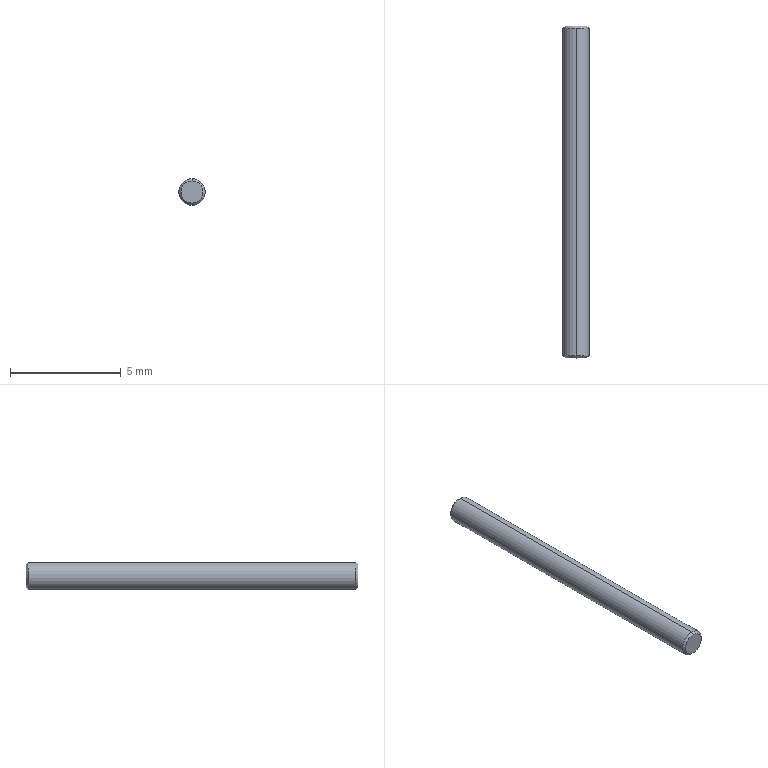Part | SolidWorks | features Chamfer 1, Extrusion 1 | 1 solid | 8 faces | box 1.2 x 15 x 1.2 mm | volume 16.929 mm3 | cone 4 | cylinder 2 | plane 2 | commonest cylinder face diameters 1.2 x2
STEP:
#1=CARTESIAN_POINT('',(0.,15.,0.5));
#2=VERTEX_POINT('',#1);
#3=CARTESIAN_POINT('',(0.,15.,-0.5));
#4=VERTEX_POINT('',#3);
#5=CARTESIAN_POINT('',(0.,15.,0.));
#6=DIRECTION('',(0.,1.,0.));
#7=DIRECTION('',(0.,0.,1.));
#8=AXIS2_PLACEMENT_3D('',#5,#6,#7);
#9=CIRCLE('',#8,0.5);
#10=EDGE_CURVE('',#2,#4,#9,.T.);
#11=ORIENTED_EDGE('',*,*,#10,.F.);
#12=CARTESIAN_POINT('',(0.,14.9,0.6));
#13=VERTEX_POINT('',#12);
#14=CARTESIAN_POINT('',(0.,15.,0.5));
#15=DIRECTION('',(0.,-0.7071,0.7071));
#16=VECTOR('',#15,1000.);
#17=LINE('',#14,#16);
#18=EDGE_CURVE('',#2,#13,#17,.T.);
#19=ORIENTED_EDGE('',*,*,#18,.T.);
#20=CARTESIAN_POINT('',(0.,14.9,-0.6));
#21=VERTEX_POINT('',#20);
#22=CARTESIAN_POINT('',(0.,14.9,0.));
#23=DIRECTION('',(0.,-1.,0.));
#24=DIRECTION('',(0.,0.,1.));
#25=AXIS2_PLACEMENT_3D('',#22,#23,#24);
#26=CIRCLE('',#25,0.6);
#27=EDGE_CURVE('',#21,#13,#26,.T.);
#28=ORIENTED_EDGE('',*,*,#27,.F.);
#29=CARTESIAN_POINT('',(0.,15.,-0.5));
#30=DIRECTION('',(0.,-0.7071,-0.7071));
#31=VECTOR('',#30,1000.);
#32=LINE('',#29,#31);
#33=EDGE_CURVE('',#4,#21,#32,.T.);
#34=ORIENTED_EDGE('',*,*,#33,.F.);
#35=EDGE_LOOP('',(#11,#19,#28,#34));
#36=FACE_OUTER_BOUND('',#35,.T.);
#37=CARTESIAN_POINT('',(0.,15.,0.));
#38=DIRECTION('',(0.,-1.,0.));
#39=DIRECTION('',(0.,0.,-1.));
#40=AXIS2_PLACEMENT_3D('',#37,#38,#39);
#41=CONICAL_SURFACE('',#40,0.5,0.7854);
#42=ADVANCED_FACE('',(#36),#41,.T.);
#43=CARTESIAN_POINT('',(0.,0.,-0.5));
#44=VERTEX_POINT('',#43);
#45=CARTESIAN_POINT('',(0.,0.,0.5));
#46=VERTEX_POINT('',#45);
#47=CARTESIAN_POINT('',(0.,0.,0.));
#48=DIRECTION('',(0.,-1.,0.));
#49=DIRECTION('',(0.,0.,1.));
#50=AXIS2_PLACEMENT_3D('',#47,#48,#49);
#51=CIRCLE('',#50,0.5);
#52=EDGE_CURVE('',#44,#46,#51,.T.);
#53=ORIENTED_EDGE('',*,*,#52,.F.);
#54=CARTESIAN_POINT('',(0.,0.1,-0.6));
#55=VERTEX_POINT('',#54);
#56=CARTESIAN_POINT('',(0.,0.1,-0.6));
#57=DIRECTION('',(0.,0.7071,-0.7071));
#58=VECTOR('',#57,1000.);
#59=LINE('',#56,#58);
#60=EDGE_CURVE('',#44,#55,#59,.T.);
#61=ORIENTED_EDGE('',*,*,#60,.T.);
#62=CARTESIAN_POINT('',(0.,0.1,0.6));
#63=VERTEX_POINT('',#62);
#64=CARTESIAN_POINT('',(0.,0.1,0.));
#65=DIRECTION('',(0.,1.,0.));
#66=DIRECTION('',(0.,0.,1.));
#67=AXIS2_PLACEMENT_3D('',#64,#65,#66);
#68=CIRCLE('',#67,0.6);
#69=EDGE_CURVE('',#63,#55,#68,.T.);
#70=ORIENTED_EDGE('',*,*,#69,.F.);
#71=CARTESIAN_POINT('',(0.,0.1,0.6));
#72=DIRECTION('',(0.,0.7071,0.7071));
#73=VECTOR('',#72,1000.);
#74=LINE('',#71,#73);
#75=EDGE_CURVE('',#46,#63,#74,.T.);
#76=ORIENTED_EDGE('',*,*,#75,.F.);
#77=EDGE_LOOP('',(#53,#61,#70,#76));
#78=FACE_OUTER_BOUND('',#77,.T.);
#79=CARTESIAN_POINT('',(0.,0.1,0.));
#80=DIRECTION('',(0.,1.,0.));
#81=DIRECTION('',(0.,0.,1.));
#82=AXIS2_PLACEMENT_3D('',#79,#80,#81);
#83=CONICAL_SURFACE('',#82,0.6,0.7854);
#84=ADVANCED_FACE('',(#78),#83,.T.);
#85=ORIENTED_EDGE('',*,*,#27,.T.);
#86=CARTESIAN_POINT('',(0.,15.,0.6));
#87=DIRECTION('',(0.,-1.,0.));
#88=VECTOR('',#87,1000.);
#89=LINE('',#86,#88);
#90=EDGE_CURVE('',#13,#63,#89,.T.);
#91=ORIENTED_EDGE('',*,*,#90,.T.);
#92=ORIENTED_EDGE('',*,*,#69,.T.);
#93=CARTESIAN_POINT('',(0.,15.,-0.6));
#94=DIRECTION('',(0.,-1.,0.));
#95=VECTOR('',#94,1000.);
#96=LINE('',#93,#95);
#97=EDGE_CURVE('',#21,#55,#96,.T.);
#98=ORIENTED_EDGE('',*,*,#97,.F.);
#99=EDGE_LOOP('',(#85,#91,#92,#98));
#100=FACE_OUTER_BOUND('',#99,.T.);
#101=CARTESIAN_POINT('',(0.,15.,0.));
#102=DIRECTION('',(0.,-1.,0.));
#103=DIRECTION('',(0.,0.,-1.));
#104=AXIS2_PLACEMENT_3D('',#101,#102,#103);
#105=CYLINDRICAL_SURFACE('',#104,0.6);
#106=ADVANCED_FACE('',(#100),#105,.T.);
#107=ORIENTED_EDGE('',*,*,#90,.F.);
#108=CARTESIAN_POINT('',(0.,14.9,0.));
#109=DIRECTION('',(0.,-1.,0.));
#110=DIRECTION('',(0.,0.,1.));
#111=AXIS2_PLACEMENT_3D('',#108,#109,#110);
#112=CIRCLE('',#111,0.6);
#113=EDGE_CURVE('',#13,#21,#112,.T.);
#114=ORIENTED_EDGE('',*,*,#113,.T.);
#115=ORIENTED_EDGE('',*,*,#97,.T.);
#116=CARTESIAN_POINT('',(0.,0.1,0.));
#117=DIRECTION('',(0.,1.,0.));
#118=DIRECTION('',(0.,0.,1.));
#119=AXIS2_PLACEMENT_3D('',#116,#117,#118);
#120=CIRCLE('',#119,0.6);
#121=EDGE_CURVE('',#55,#63,#120,.T.);
#122=ORIENTED_EDGE('',*,*,#121,.T.);
#123=EDGE_LOOP('',(#107,#114,#115,#122));
#124=FACE_OUTER_BOUND('',#123,.T.);
#125=CARTESIAN_POINT('',(0.,15.,0.));
#126=DIRECTION('',(0.,-1.,0.));
#127=DIRECTION('',(0.,0.,-1.));
#128=AXIS2_PLACEMENT_3D('',#125,#126,#127);
#129=CYLINDRICAL_SURFACE('',#128,0.6);
#130=ADVANCED_FACE('',(#124),#129,.T.);
#131=CARTESIAN_POINT('',(0.,15.,0.));
#132=DIRECTION('',(0.,1.,0.));
#133=DIRECTION('',(0.,0.,1.));
#134=AXIS2_PLACEMENT_3D('',#131,#132,#133);
#135=CIRCLE('',#134,0.5);
#136=EDGE_CURVE('',#4,#2,#135,.T.);
#137=ORIENTED_EDGE('',*,*,#136,.T.);
#138=ORIENTED_EDGE('',*,*,#10,.T.);
#139=EDGE_LOOP('',(#137,#138));
#140=FACE_OUTER_BOUND('',#139,.T.);
#141=CARTESIAN_POINT('',(0.,15.,0.));
#142=DIRECTION('',(0.,1.,0.));
#143=DIRECTION('',(0.,0.,1.));
#144=AXIS2_PLACEMENT_3D('',#141,#142,#143);
#145=PLANE('',#144);
#146=ADVANCED_FACE('',(#140),#145,.T.);
#147=CARTESIAN_POINT('',(0.,0.,0.));
#148=DIRECTION('',(0.,-1.,0.));
#149=DIRECTION('',(0.,0.,1.));
#150=AXIS2_PLACEMENT_3D('',#147,#148,#149);
#151=CIRCLE('',#150,0.5);
#152=EDGE_CURVE('',#46,#44,#151,.T.);
#153=ORIENTED_EDGE('',*,*,#152,.T.);
#154=ORIENTED_EDGE('',*,*,#52,.T.);
#155=EDGE_LOOP('',(#153,#154));
#156=FACE_OUTER_BOUND('',#155,.T.);
#157=CARTESIAN_POINT('',(0.,0.,0.));
#158=DIRECTION('',(0.,1.,0.));
#159=DIRECTION('',(0.,0.,1.));
#160=AXIS2_PLACEMENT_3D('',#157,#158,#159);
#161=PLANE('',#160);
#162=ADVANCED_FACE('',(#156),#161,.F.);
#163=ORIENTED_EDGE('',*,*,#60,.F.);
#164=ORIENTED_EDGE('',*,*,#152,.F.);
#165=ORIENTED_EDGE('',*,*,#75,.T.);
#166=ORIENTED_EDGE('',*,*,#121,.F.);
#167=EDGE_LOOP('',(#163,#164,#165,#166));
#168=FACE_OUTER_BOUND('',#167,.T.);
#169=CARTESIAN_POINT('',(0.,0.1,0.));
#170=DIRECTION('',(0.,1.,0.));
#171=DIRECTION('',(0.,0.,1.));
#172=AXIS2_PLACEMENT_3D('',#169,#170,#171);
#173=CONICAL_SURFACE('',#172,0.6,0.7854);
#174=ADVANCED_FACE('',(#168),#173,.T.);
#175=ORIENTED_EDGE('',*,*,#18,.F.);
#176=ORIENTED_EDGE('',*,*,#136,.F.);
#177=ORIENTED_EDGE('',*,*,#33,.T.);
#178=ORIENTED_EDGE('',*,*,#113,.F.);
#179=EDGE_LOOP('',(#175,#176,#177,#178));
#180=FACE_OUTER_BOUND('',#179,.T.);
#181=CARTESIAN_POINT('',(0.,15.,0.));
#182=DIRECTION('',(0.,-1.,0.));
#183=DIRECTION('',(0.,0.,-1.));
#184=AXIS2_PLACEMENT_3D('',#181,#182,#183);
#185=CONICAL_SURFACE('',#184,0.5,0.7854);
#186=ADVANCED_FACE('',(#180),#185,.T.);
#187=CLOSED_SHELL('',(#42,#84,#106,#130,#146,#162,#174,#186));
#188=MANIFOLD_SOLID_BREP('',#187);
#189=CARTESIAN_POINT('',(0.,0.,0.));
#190=DIRECTION('',(0.,0.,1.));
#191=DIRECTION('',(1.,0.,0.));
#192=AXIS2_PLACEMENT_3D('',#189,#190,#191);
#193=(LENGTH_UNIT()NAMED_UNIT(*)SI_UNIT(.MILLI.,.METRE.));
#194=UNCERTAINTY_MEASURE_WITH_UNIT(LENGTH_MEASURE(0.00001),#193,'','');
#195=(NAMED_UNIT(*)PLANE_ANGLE_UNIT()SI_UNIT($,.RADIAN.));
#196=(NAMED_UNIT(*)SI_UNIT($,.STERADIAN.)SOLID_ANGLE_UNIT());
#197=(GEOMETRIC_REPRESENTATION_CONTEXT(3)GLOBAL_UNCERTAINTY_ASSIGNED_CONTEXT((#194))GLOBAL_UNIT_ASSIGNED_CONTEXT((#193,#195,#196))REPRESENTATION_CONTEXT('',''));
#198=ADVANCED_BREP_SHAPE_REPRESENTATION('',(#188,#192),#197);